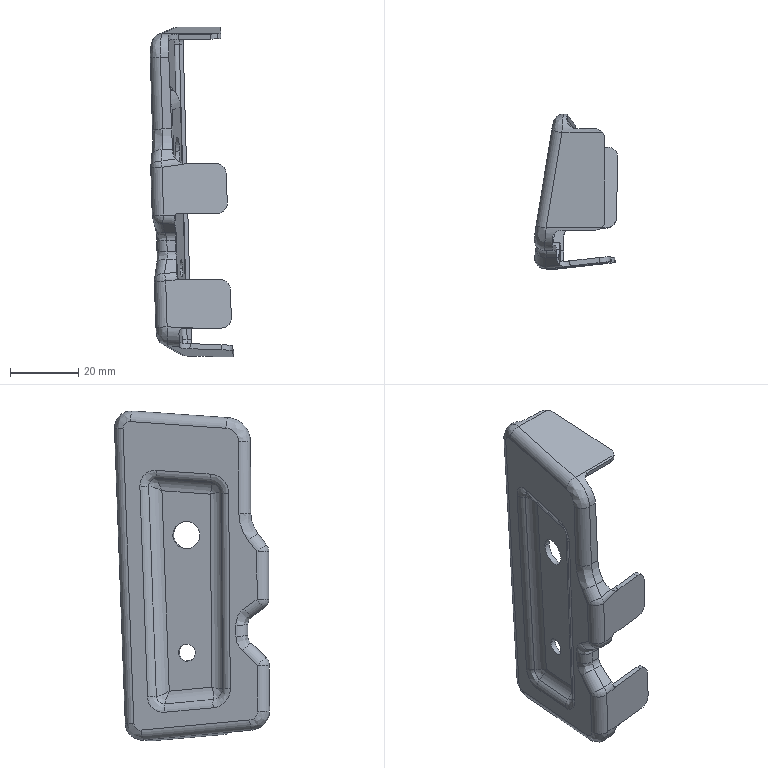Part | 1 solid | 172 faces | box 24.547 x 45.547 x 96.871 mm | volume 8744 mm3 | spline 89 | cylinder 50 | plane 20 | other 7 | sphere 6 | commonest cylinder face diameters 3 x17 6 x17 9 x4 12 x4 7 x2 10 x2